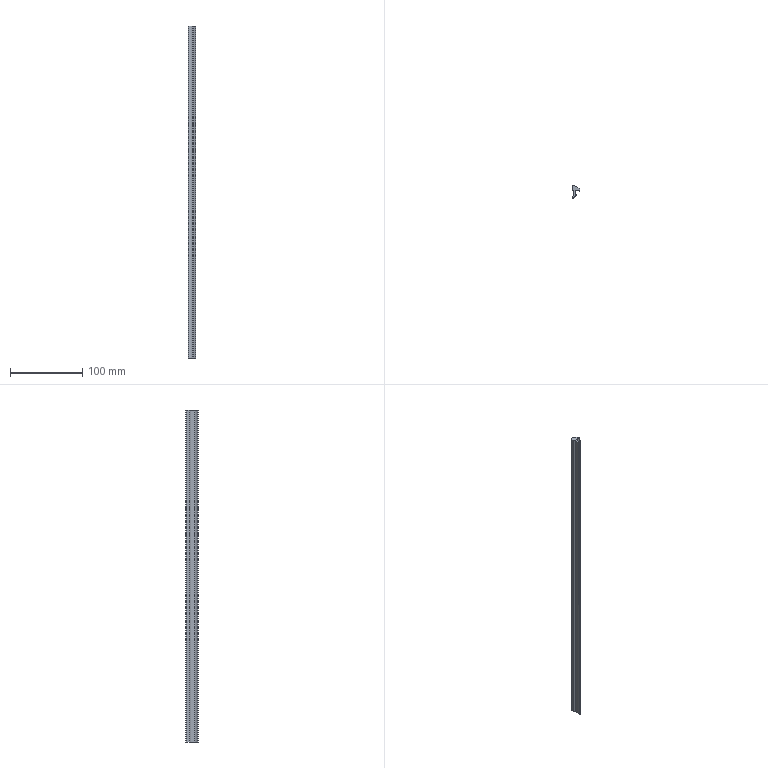Part | SolidWorks | features BaseBody 1, MoveFace 1 | 1 solid | 20 faces | box 10.8 x 17.5 x 461 mm | volume 36327 mm3 | cylinder 11 | plane 9 | commonest cylinder face diameters 1.6 x2 14 x2 0.4 x1 0.6 x1 0.8 x1 2.6 x1
STEP:
#1=CARTESIAN_POINT('',(-3.236,-11.055,361.));
#2=VERTEX_POINT('',#1);
#3=CARTESIAN_POINT('',(-4.3,-10.3,361.));
#4=VERTEX_POINT('',#3);
#5=CARTESIAN_POINT('',(-3.5,-10.3,361.));
#6=DIRECTION('',(0.,0.,-1.));
#7=DIRECTION('',(1.,0.,0.));
#8=AXIS2_PLACEMENT_3D('',#5,#6,#7);
#9=CIRCLE('',#8,0.8);
#10=EDGE_CURVE('',#2,#4,#9,.T.);
#11=ORIENTED_EDGE('',*,*,#10,.T.);
#12=CARTESIAN_POINT('',(-4.3,-10.3,-100.));
#13=VERTEX_POINT('',#12);
#14=CARTESIAN_POINT('',(-4.3,-10.3,-100.));
#15=DIRECTION('',(0.,0.,-1.));
#16=VECTOR('',#15,1000.);
#17=LINE('',#14,#16);
#18=EDGE_CURVE('',#4,#13,#17,.T.);
#19=ORIENTED_EDGE('',*,*,#18,.T.);
#20=CARTESIAN_POINT('',(-3.236,-11.055,-100.));
#21=VERTEX_POINT('',#20);
#22=CARTESIAN_POINT('',(-3.5,-10.3,-100.));
#23=DIRECTION('',(0.,0.,1.));
#24=DIRECTION('',(-1.,0.,0.));
#25=AXIS2_PLACEMENT_3D('',#22,#23,#24);
#26=CIRCLE('',#25,0.8);
#27=EDGE_CURVE('',#13,#21,#26,.T.);
#28=ORIENTED_EDGE('',*,*,#27,.T.);
#29=CARTESIAN_POINT('',(-3.236,-11.055,-100.));
#30=DIRECTION('',(0.,0.,-1.));
#31=VECTOR('',#30,1000.);
#32=LINE('',#29,#31);
#33=EDGE_CURVE('',#2,#21,#32,.T.);
#34=ORIENTED_EDGE('',*,*,#33,.F.);
#35=EDGE_LOOP('',(#11,#19,#28,#34));
#36=FACE_OUTER_BOUND('',#35,.T.);
#37=CARTESIAN_POINT('',(-3.5,-10.3,-100.));
#38=DIRECTION('',(0.,0.,-1.));
#39=DIRECTION('',(-1.,0.,0.));
#40=AXIS2_PLACEMENT_3D('',#37,#38,#39);
#41=CYLINDRICAL_SURFACE('',#40,0.8);
#42=ADVANCED_FACE('',(#36),#41,.T.);
#43=CARTESIAN_POINT('',(1.184,-6.397,-100.));
#44=VERTEX_POINT('',#43);
#45=CARTESIAN_POINT('',(-5.702,-4.29,-100.));
#46=DIRECTION('',(0.,0.,1.));
#47=DIRECTION('',(-1.,0.,0.));
#48=AXIS2_PLACEMENT_3D('',#45,#46,#47);
#49=CIRCLE('',#48,7.201);
#50=EDGE_CURVE('',#21,#44,#49,.T.);
#51=ORIENTED_EDGE('',*,*,#50,.T.);
#52=CARTESIAN_POINT('',(1.184,-6.397,361.));
#53=VERTEX_POINT('',#52);
#54=CARTESIAN_POINT('',(1.184,-6.397,-100.));
#55=DIRECTION('',(0.,0.,1.));
#56=VECTOR('',#55,1000.);
#57=LINE('',#54,#56);
#58=EDGE_CURVE('',#44,#53,#57,.T.);
#59=ORIENTED_EDGE('',*,*,#58,.T.);
#60=CARTESIAN_POINT('',(-5.702,-4.29,361.));
#61=DIRECTION('',(0.,0.,-1.));
#62=DIRECTION('',(1.,0.,0.));
#63=AXIS2_PLACEMENT_3D('',#60,#61,#62);
#64=CIRCLE('',#63,7.201);
#65=EDGE_CURVE('',#53,#2,#64,.T.);
#66=ORIENTED_EDGE('',*,*,#65,.T.);
#67=ORIENTED_EDGE('',*,*,#33,.T.);
#68=EDGE_LOOP('',(#51,#59,#66,#67));
#69=FACE_OUTER_BOUND('',#68,.T.);
#70=CARTESIAN_POINT('',(-5.702,-4.29,-100.));
#71=DIRECTION('',(0.,0.,-1.));
#72=DIRECTION('',(-1.,0.,0.));
#73=AXIS2_PLACEMENT_3D('',#70,#71,#72);
#74=CYLINDRICAL_SURFACE('',#73,7.201);
#75=ADVANCED_FACE('',(#69),#74,.T.);
#76=CARTESIAN_POINT('',(0.9,-6.,-100.));
#77=VERTEX_POINT('',#76);
#78=CARTESIAN_POINT('',(0.9,-6.3,-100.));
#79=DIRECTION('',(0.,0.,1.));
#80=DIRECTION('',(-1.,0.,0.));
#81=AXIS2_PLACEMENT_3D('',#78,#79,#80);
#82=CIRCLE('',#81,0.3);
#83=EDGE_CURVE('',#44,#77,#82,.T.);
#84=ORIENTED_EDGE('',*,*,#83,.T.);
#85=CARTESIAN_POINT('',(0.9,-6.,361.));
#86=VERTEX_POINT('',#85);
#87=CARTESIAN_POINT('',(0.9,-6.,-100.));
#88=DIRECTION('',(0.,0.,1.));
#89=VECTOR('',#88,1000.);
#90=LINE('',#87,#89);
#91=EDGE_CURVE('',#77,#86,#90,.T.);
#92=ORIENTED_EDGE('',*,*,#91,.T.);
#93=CARTESIAN_POINT('',(0.9,-6.3,361.));
#94=DIRECTION('',(0.,0.,-1.));
#95=DIRECTION('',(1.,0.,0.));
#96=AXIS2_PLACEMENT_3D('',#93,#94,#95);
#97=CIRCLE('',#96,0.3);
#98=EDGE_CURVE('',#86,#53,#97,.T.);
#99=ORIENTED_EDGE('',*,*,#98,.T.);
#100=ORIENTED_EDGE('',*,*,#58,.F.);
#101=EDGE_LOOP('',(#84,#92,#99,#100));
#102=FACE_OUTER_BOUND('',#101,.T.);
#103=CARTESIAN_POINT('',(0.9,-6.3,-100.));
#104=DIRECTION('',(0.,0.,-1.));
#105=DIRECTION('',(-1.,0.,0.));
#106=AXIS2_PLACEMENT_3D('',#103,#104,#105);
#107=CYLINDRICAL_SURFACE('',#106,0.3);
#108=ADVANCED_FACE('',(#102),#107,.T.);
#109=CARTESIAN_POINT('',(-2.5,-0.5,-100.));
#110=VERTEX_POINT('',#109);
#111=CARTESIAN_POINT('',(-2.5,-6.153,-100.));
#112=VERTEX_POINT('',#111);
#113=CARTESIAN_POINT('',(-2.5,-6.397,-100.));
#114=DIRECTION('',(0.,-1.,0.));
#115=VECTOR('',#114,1000.);
#116=LINE('',#113,#115);
#117=EDGE_CURVE('',#110,#112,#116,.T.);
#118=ORIENTED_EDGE('',*,*,#117,.F.);
#119=CARTESIAN_POINT('',(-4.2,1.695,-100.));
#120=VERTEX_POINT('',#119);
#121=CARTESIAN_POINT('',(-1.701,1.875,-100.));
#122=DIRECTION('',(0.,0.,1.));
#123=DIRECTION('',(-1.,0.,0.));
#124=AXIS2_PLACEMENT_3D('',#121,#122,#123);
#125=CIRCLE('',#124,2.506);
#126=EDGE_CURVE('',#120,#110,#125,.T.);
#127=ORIENTED_EDGE('',*,*,#126,.F.);
#128=CARTESIAN_POINT('',(-4.2,5.1,-100.));
#129=VERTEX_POINT('',#128);
#130=CARTESIAN_POINT('',(-4.2,-6.397,-100.));
#131=DIRECTION('',(0.,-1.,0.));
#132=VECTOR('',#131,1000.);
#133=LINE('',#130,#132);
#134=EDGE_CURVE('',#129,#120,#133,.T.);
#135=ORIENTED_EDGE('',*,*,#134,.F.);
#136=CARTESIAN_POINT('',(-2.892,6.4,-100.));
#137=VERTEX_POINT('',#136);
#138=CARTESIAN_POINT('',(-2.9,5.1,-100.));
#139=DIRECTION('',(0.,0.,1.));
#140=DIRECTION('',(-1.,0.,0.));
#141=AXIS2_PLACEMENT_3D('',#138,#139,#140);
#142=CIRCLE('',#141,1.3);
#143=EDGE_CURVE('',#137,#129,#142,.T.);
#144=ORIENTED_EDGE('',*,*,#143,.F.);
#145=CARTESIAN_POINT('',(0.5,5.5,-100.));
#146=VERTEX_POINT('',#145);
#147=CARTESIAN_POINT('',(-2.934,-0.5999,-100.));
#148=DIRECTION('',(0.,0.,1.));
#149=DIRECTION('',(-1.,0.,0.));
#150=AXIS2_PLACEMENT_3D('',#147,#148,#149);
#151=CIRCLE('',#150,7.);
#152=EDGE_CURVE('',#146,#137,#151,.T.);
#153=ORIENTED_EDGE('',*,*,#152,.F.);
#154=CARTESIAN_POINT('',(5.5,1.7,-100.));
#155=VERTEX_POINT('',#154);
#156=CARTESIAN_POINT('',(5.5,1.7,-100.));
#157=DIRECTION('',(-0.7962,0.6051,0.));
#158=VECTOR('',#157,1000.);
#159=LINE('',#156,#158);
#160=EDGE_CURVE('',#155,#146,#159,.T.);
#161=ORIENTED_EDGE('',*,*,#160,.F.);
#162=CARTESIAN_POINT('',(6.458,-0.2215,-100.));
#163=VERTEX_POINT('',#162);
#164=CARTESIAN_POINT('',(6.458,-0.2215,-100.));
#165=DIRECTION('',(-0.4462,0.8949,0.));
#166=VECTOR('',#165,1000.);
#167=LINE('',#164,#166);
#168=EDGE_CURVE('',#163,#155,#167,.T.);
#169=ORIENTED_EDGE('',*,*,#168,.F.);
#170=CARTESIAN_POINT('',(5.895,-0.7433,-100.));
#171=VERTEX_POINT('',#170);
#172=CARTESIAN_POINT('',(6.1,-0.4,-100.));
#173=DIRECTION('',(0.,0.,1.));
#174=DIRECTION('',(-1.,0.,0.));
#175=AXIS2_PLACEMENT_3D('',#172,#173,#174);
#176=CIRCLE('',#175,0.4);
#177=EDGE_CURVE('',#171,#163,#176,.T.);
#178=ORIENTED_EDGE('',*,*,#177,.F.);
#179=CARTESIAN_POINT('',(3.,0.,-100.));
#180=VERTEX_POINT('',#179);
#181=CARTESIAN_POINT('',(2.746,-6.995,-100.));
#182=DIRECTION('',(0.,0.,-1.));
#183=DIRECTION('',(-1.,0.,0.));
#184=AXIS2_PLACEMENT_3D('',#181,#182,#183);
#185=CIRCLE('',#184,7.);
#186=EDGE_CURVE('',#180,#171,#185,.T.);
#187=ORIENTED_EDGE('',*,*,#186,.F.);
#188=CARTESIAN_POINT('',(0.,0.,-100.));
#189=VERTEX_POINT('',#188);
#190=CARTESIAN_POINT('',(-6.814,0.,-100.));
#191=DIRECTION('',(1.,0.,0.));
#192=VECTOR('',#191,1000.);
#193=LINE('',#190,#192);
#194=EDGE_CURVE('',#189,#180,#193,.T.);
#195=ORIENTED_EDGE('',*,*,#194,.F.);
#196=CARTESIAN_POINT('',(0.,-5.8,-100.));
#197=VERTEX_POINT('',#196);
#198=CARTESIAN_POINT('',(0.,-6.397,-100.));
#199=DIRECTION('',(0.,1.,0.));
#200=VECTOR('',#199,1000.);
#201=LINE('',#198,#200);
#202=EDGE_CURVE('',#197,#189,#201,.T.);
#203=ORIENTED_EDGE('',*,*,#202,.F.);
#204=CARTESIAN_POINT('',(0.2,-6.,-100.));
#205=VERTEX_POINT('',#204);
#206=CARTESIAN_POINT('',(0.2,-5.8,-100.));
#207=DIRECTION('',(0.,0.,1.));
#208=DIRECTION('',(-1.,0.,0.));
#209=AXIS2_PLACEMENT_3D('',#206,#207,#208);
#210=CIRCLE('',#209,0.2);
#211=EDGE_CURVE('',#197,#205,#210,.T.);
#212=ORIENTED_EDGE('',*,*,#211,.T.);
#213=CARTESIAN_POINT('',(-6.814,-6.,-100.));
#214=DIRECTION('',(-1.,0.,0.));
#215=VECTOR('',#214,1000.);
#216=LINE('',#213,#215);
#217=EDGE_CURVE('',#77,#205,#216,.T.);
#218=ORIENTED_EDGE('',*,*,#217,.F.);
#219=ORIENTED_EDGE('',*,*,#83,.F.);
#220=ORIENTED_EDGE('',*,*,#50,.F.);
#221=ORIENTED_EDGE('',*,*,#27,.F.);
#222=CARTESIAN_POINT('',(-3.998,-9.674,-100.));
#223=VERTEX_POINT('',#222);
#224=CARTESIAN_POINT('',(-3.5,-10.3,-100.));
#225=DIRECTION('',(0.,0.,1.));
#226=DIRECTION('',(-1.,0.,0.));
#227=AXIS2_PLACEMENT_3D('',#224,#225,#226);
#228=CIRCLE('',#227,0.8);
#229=EDGE_CURVE('',#223,#13,#228,.T.);
#230=ORIENTED_EDGE('',*,*,#229,.F.);
#231=CARTESIAN_POINT('',(-6.814,-6.397,-100.));
#232=DIRECTION('',(0.,0.,-1.));
#233=DIRECTION('',(-1.,0.,0.));
#234=AXIS2_PLACEMENT_3D('',#231,#232,#233);
#235=CIRCLE('',#234,4.321);
#236=EDGE_CURVE('',#112,#223,#235,.T.);
#237=ORIENTED_EDGE('',*,*,#236,.F.);
#238=EDGE_LOOP('',(#118,#127,#135,#144,#153,#161,#169,#178,#187,#195,#203,#212,#218,#219,#220,#221,#230,#237));
#239=FACE_OUTER_BOUND('',#238,.T.);
#240=CARTESIAN_POINT('',(-6.814,-6.397,-100.));
#241=DIRECTION('',(0.,0.,1.));
#242=DIRECTION('',(1.,0.,0.));
#243=AXIS2_PLACEMENT_3D('',#240,#241,#242);
#244=PLANE('',#243);
#245=ADVANCED_FACE('',(#239),#244,.F.);
#246=ORIENTED_EDGE('',*,*,#18,.F.);
#247=CARTESIAN_POINT('',(-3.998,-9.674,361.));
#248=VERTEX_POINT('',#247);
#249=CARTESIAN_POINT('',(-3.5,-10.3,361.));
#250=DIRECTION('',(0.,0.,-1.));
#251=DIRECTION('',(1.,0.,0.));
#252=AXIS2_PLACEMENT_3D('',#249,#250,#251);
#253=CIRCLE('',#252,0.8);
#254=EDGE_CURVE('',#4,#248,#253,.T.);
#255=ORIENTED_EDGE('',*,*,#254,.T.);
#256=CARTESIAN_POINT('',(-3.998,-9.674,-100.));
#257=DIRECTION('',(0.,0.,-1.));
#258=VECTOR('',#257,1000.);
#259=LINE('',#256,#258);
#260=EDGE_CURVE('',#248,#223,#259,.T.);
#261=ORIENTED_EDGE('',*,*,#260,.T.);
#262=ORIENTED_EDGE('',*,*,#229,.T.);
#263=EDGE_LOOP('',(#246,#255,#261,#262));
#264=FACE_OUTER_BOUND('',#263,.T.);
#265=CARTESIAN_POINT('',(-3.5,-10.3,-100.));
#266=DIRECTION('',(0.,0.,-1.));
#267=DIRECTION('',(-1.,0.,0.));
#268=AXIS2_PLACEMENT_3D('',#265,#266,#267);
#269=CYLINDRICAL_SURFACE('',#268,0.8);
#270=ADVANCED_FACE('',(#264),#269,.T.);
#271=CARTESIAN_POINT('',(-4.2,1.695,361.));
#272=VERTEX_POINT('',#271);
#273=CARTESIAN_POINT('',(-2.5,-0.5,361.));
#274=VERTEX_POINT('',#273);
#275=CARTESIAN_POINT('',(-1.701,1.875,361.));
#276=DIRECTION('',(0.,0.,1.));
#277=DIRECTION('',(1.,0.,0.));
#278=AXIS2_PLACEMENT_3D('',#275,#276,#277);
#279=CIRCLE('',#278,2.506);
#280=EDGE_CURVE('',#272,#274,#279,.T.);
#281=ORIENTED_EDGE('',*,*,#280,.T.);
#282=CARTESIAN_POINT('',(-2.5,-6.153,361.));
#283=VERTEX_POINT('',#282);
#284=CARTESIAN_POINT('',(-2.5,-6.397,361.));
#285=DIRECTION('',(0.,-1.,0.));
#286=VECTOR('',#285,1000.);
#287=LINE('',#284,#286);
#288=EDGE_CURVE('',#274,#283,#287,.T.);
#289=ORIENTED_EDGE('',*,*,#288,.T.);
#290=CARTESIAN_POINT('',(-6.814,-6.397,361.));
#291=DIRECTION('',(0.,0.,-1.));
#292=DIRECTION('',(1.,0.,0.));
#293=AXIS2_PLACEMENT_3D('',#290,#291,#292);
#294=CIRCLE('',#293,4.321);
#295=EDGE_CURVE('',#283,#248,#294,.T.);
#296=ORIENTED_EDGE('',*,*,#295,.T.);
#297=ORIENTED_EDGE('',*,*,#254,.F.);
#298=ORIENTED_EDGE('',*,*,#10,.F.);
#299=ORIENTED_EDGE('',*,*,#65,.F.);
#300=ORIENTED_EDGE('',*,*,#98,.F.);
#301=CARTESIAN_POINT('',(0.2,-6.,361.));
#302=VERTEX_POINT('',#301);
#303=CARTESIAN_POINT('',(-6.814,-6.,361.));
#304=DIRECTION('',(-1.,0.,0.));
#305=VECTOR('',#304,1000.);
#306=LINE('',#303,#305);
#307=EDGE_CURVE('',#86,#302,#306,.T.);
#308=ORIENTED_EDGE('',*,*,#307,.T.);
#309=CARTESIAN_POINT('',(0.,-5.8,361.));
#310=VERTEX_POINT('',#309);
#311=CARTESIAN_POINT('',(0.2,-5.8,361.));
#312=DIRECTION('',(0.,0.,-1.));
#313=DIRECTION('',(1.,0.,0.));
#314=AXIS2_PLACEMENT_3D('',#311,#312,#313);
#315=CIRCLE('',#314,0.2);
#316=EDGE_CURVE('',#302,#310,#315,.T.);
#317=ORIENTED_EDGE('',*,*,#316,.T.);
#318=CARTESIAN_POINT('',(0.,0.,361.));
#319=VERTEX_POINT('',#318);
#320=CARTESIAN_POINT('',(0.,-6.397,361.));
#321=DIRECTION('',(0.,1.,0.));
#322=VECTOR('',#321,1000.);
#323=LINE('',#320,#322);
#324=EDGE_CURVE('',#310,#319,#323,.T.);
#325=ORIENTED_EDGE('',*,*,#324,.T.);
#326=CARTESIAN_POINT('',(3.,0.,361.));
#327=VERTEX_POINT('',#326);
#328=CARTESIAN_POINT('',(-6.814,0.,361.));
#329=DIRECTION('',(1.,0.,0.));
#330=VECTOR('',#329,1000.);
#331=LINE('',#328,#330);
#332=EDGE_CURVE('',#319,#327,#331,.T.);
#333=ORIENTED_EDGE('',*,*,#332,.T.);
#334=CARTESIAN_POINT('',(5.895,-0.7433,361.));
#335=VERTEX_POINT('',#334);
#336=CARTESIAN_POINT('',(2.746,-6.995,361.));
#337=DIRECTION('',(0.,0.,-1.));
#338=DIRECTION('',(1.,0.,0.));
#339=AXIS2_PLACEMENT_3D('',#336,#337,#338);
#340=CIRCLE('',#339,7.);
#341=EDGE_CURVE('',#327,#335,#340,.T.);
#342=ORIENTED_EDGE('',*,*,#341,.T.);
#343=CARTESIAN_POINT('',(6.458,-0.2215,361.));
#344=VERTEX_POINT('',#343);
#345=CARTESIAN_POINT('',(6.1,-0.4,361.));
#346=DIRECTION('',(0.,0.,-1.));
#347=DIRECTION('',(1.,0.,0.));
#348=AXIS2_PLACEMENT_3D('',#345,#346,#347);
#349=CIRCLE('',#348,0.4);
#350=EDGE_CURVE('',#344,#335,#349,.T.);
#351=ORIENTED_EDGE('',*,*,#350,.F.);
#352=CARTESIAN_POINT('',(5.5,1.7,361.));
#353=VERTEX_POINT('',#352);
#354=CARTESIAN_POINT('',(6.282,0.1323,361.));
#355=DIRECTION('',(-0.4462,0.8949,0.));
#356=VECTOR('',#355,1000.);
#357=LINE('',#354,#356);
#358=EDGE_CURVE('',#344,#353,#357,.T.);
#359=ORIENTED_EDGE('',*,*,#358,.T.);
#360=CARTESIAN_POINT('',(0.5,5.5,361.));
#361=VERTEX_POINT('',#360);
#362=CARTESIAN_POINT('',(1.595,4.668,361.));
#363=DIRECTION('',(-0.7962,0.6051,0.));
#364=VECTOR('',#363,1000.);
#365=LINE('',#362,#364);
#366=EDGE_CURVE('',#353,#361,#365,.T.);
#367=ORIENTED_EDGE('',*,*,#366,.T.);
#368=CARTESIAN_POINT('',(-2.892,6.4,361.));
#369=VERTEX_POINT('',#368);
#370=CARTESIAN_POINT('',(-2.934,-0.5999,361.));
#371=DIRECTION('',(0.,0.,1.));
#372=DIRECTION('',(1.,0.,0.));
#373=AXIS2_PLACEMENT_3D('',#370,#371,#372);
#374=CIRCLE('',#373,7.);
#375=EDGE_CURVE('',#361,#369,#374,.T.);
#376=ORIENTED_EDGE('',*,*,#375,.T.);
#377=CARTESIAN_POINT('',(-4.2,5.1,361.));
#378=VERTEX_POINT('',#377);
#379=CARTESIAN_POINT('',(-2.9,5.1,361.));
#380=DIRECTION('',(0.,0.,1.));
#381=DIRECTION('',(1.,0.,0.));
#382=AXIS2_PLACEMENT_3D('',#379,#380,#381);
#383=CIRCLE('',#382,1.3);
#384=EDGE_CURVE('',#369,#378,#383,.T.);
#385=ORIENTED_EDGE('',*,*,#384,.T.);
#386=CARTESIAN_POINT('',(-4.2,-6.397,361.));
#387=DIRECTION('',(0.,-1.,0.));
#388=VECTOR('',#387,1000.);
#389=LINE('',#386,#388);
#390=EDGE_CURVE('',#378,#272,#389,.T.);
#391=ORIENTED_EDGE('',*,*,#390,.T.);
#392=EDGE_LOOP('',(#281,#289,#296,#297,#298,#299,#300,#308,#317,#325,#333,#342,#351,#359,#367,#376,#385,#391));
#393=FACE_OUTER_BOUND('',#392,.T.);
#394=CARTESIAN_POINT('',(-6.814,-6.397,361.));
#395=DIRECTION('',(0.,0.,1.));
#396=DIRECTION('',(1.,0.,0.));
#397=AXIS2_PLACEMENT_3D('',#394,#395,#396);
#398=PLANE('',#397);
#399=ADVANCED_FACE('',(#393),#398,.T.);
#400=ORIENTED_EDGE('',*,*,#217,.T.);
#401=CARTESIAN_POINT('',(0.2,-6.,-100.));
#402=DIRECTION('',(0.,0.,1.));
#403=VECTOR('',#402,1000.);
#404=LINE('',#401,#403);
#405=EDGE_CURVE('',#205,#302,#404,.T.);
#406=ORIENTED_EDGE('',*,*,#405,.T.);
#407=ORIENTED_EDGE('',*,*,#307,.F.);
#408=ORIENTED_EDGE('',*,*,#91,.F.);
#409=EDGE_LOOP('',(#400,#406,#407,#408));
#410=FACE_OUTER_BOUND('',#409,.T.);
#411=CARTESIAN_POINT('',(0.9,-6.,-100.));
#412=DIRECTION('',(0.,1.,0.));
#413=DIRECTION('',(0.,0.,1.));
#414=AXIS2_PLACEMENT_3D('',#411,#412,#413);
#415=PLANE('',#414);
#416=ADVANCED_FACE('',(#410),#415,.T.);
#417=CARTESIAN_POINT('',(-2.5,-6.153,-100.));
#418=DIRECTION('',(0.,0.,1.));
#419=VECTOR('',#418,1000.);
#420=LINE('',#417,#419);
#421=EDGE_CURVE('',#112,#283,#420,.T.);
#422=ORIENTED_EDGE('',*,*,#421,.F.);
#423=ORIENTED_EDGE('',*,*,#236,.T.);
#424=ORIENTED_EDGE('',*,*,#260,.F.);
#425=ORIENTED_EDGE('',*,*,#295,.F.);
#426=EDGE_LOOP('',(#422,#423,#424,#425));
#427=FACE_OUTER_BOUND('',#426,.T.);
#428=CARTESIAN_POINT('',(-6.814,-6.397,-100.));
#429=DIRECTION('',(0.,0.,-1.));
#430=DIRECTION('',(-1.,0.,0.));
#431=AXIS2_PLACEMENT_3D('',#428,#429,#430);
#432=CYLINDRICAL_SURFACE('',#431,4.321);
#433=ADVANCED_FACE('',(#427),#432,.F.);
#434=ORIENTED_EDGE('',*,*,#117,.T.);
#435=ORIENTED_EDGE('',*,*,#421,.T.);
#436=ORIENTED_EDGE('',*,*,#288,.F.);
#437=CARTESIAN_POINT('',(-2.5,-0.5,-100.));
#438=DIRECTION('',(0.,0.,-1.));
#439=VECTOR('',#438,1000.);
#440=LINE('',#437,#439);
#441=EDGE_CURVE('',#274,#110,#440,.T.);
#442=ORIENTED_EDGE('',*,*,#441,.T.);
#443=EDGE_LOOP('',(#434,#435,#436,#442));
#444=FACE_OUTER_BOUND('',#443,.T.);
#445=CARTESIAN_POINT('',(-2.5,-0.5,-100.));
#446=DIRECTION('',(-1.,0.,0.));
#447=DIRECTION('',(0.,0.,1.));
#448=AXIS2_PLACEMENT_3D('',#445,#446,#447);
#449=PLANE('',#448);
#450=ADVANCED_FACE('',(#444),#449,.T.);
#451=ORIENTED_EDGE('',*,*,#126,.T.);
#452=ORIENTED_EDGE('',*,*,#441,.F.);
#453=ORIENTED_EDGE('',*,*,#280,.F.);
#454=CARTESIAN_POINT('',(-4.2,1.695,-100.));
#455=DIRECTION('',(0.,0.,-1.));
#456=VECTOR('',#455,1000.);
#457=LINE('',#454,#456);
#458=EDGE_CURVE('',#272,#120,#457,.T.);
#459=ORIENTED_EDGE('',*,*,#458,.T.);
#460=EDGE_LOOP('',(#451,#452,#453,#459));
#461=FACE_OUTER_BOUND('',#460,.T.);
#462=CARTESIAN_POINT('',(-1.701,1.875,-100.));
#463=DIRECTION('',(0.,0.,-1.));
#464=DIRECTION('',(-1.,0.,0.));
#465=AXIS2_PLACEMENT_3D('',#462,#463,#464);
#466=CYLINDRICAL_SURFACE('',#465,2.506);
#467=ADVANCED_FACE('',(#461),#466,.T.);
#468=ORIENTED_EDGE('',*,*,#134,.T.);
#469=ORIENTED_EDGE('',*,*,#458,.F.);
#470=ORIENTED_EDGE('',*,*,#390,.F.);
#471=CARTESIAN_POINT('',(-4.2,5.1,-100.));
#472=DIRECTION('',(0.,0.,-1.));
#473=VECTOR('',#472,1000.);
#474=LINE('',#471,#473);
#475=EDGE_CURVE('',#378,#129,#474,.T.);
#476=ORIENTED_EDGE('',*,*,#475,.T.);
#477=EDGE_LOOP('',(#468,#469,#470,#476));
#478=FACE_OUTER_BOUND('',#477,.T.);
#479=CARTESIAN_POINT('',(-4.2,5.1,-100.));
#480=DIRECTION('',(-1.,0.,0.));
#481=DIRECTION('',(0.,0.,1.));
#482=AXIS2_PLACEMENT_3D('',#479,#480,#481);
#483=PLANE('',#482);
#484=ADVANCED_FACE('',(#478),#483,.T.);
#485=ORIENTED_EDGE('',*,*,#143,.T.);
#486=ORIENTED_EDGE('',*,*,#475,.F.);
#487=ORIENTED_EDGE('',*,*,#384,.F.);
#488=CARTESIAN_POINT('',(-2.892,6.4,-100.));
#489=DIRECTION('',(0.,0.,-1.));
#490=VECTOR('',#489,1000.);
#491=LINE('',#488,#490);
#492=EDGE_CURVE('',#369,#137,#491,.T.);
#493=ORIENTED_EDGE('',*,*,#492,.T.);
#494=EDGE_LOOP('',(#485,#486,#487,#493));
#495=FACE_OUTER_BOUND('',#494,.T.);
#496=CARTESIAN_POINT('',(-2.9,5.1,-100.));
#497=DIRECTION('',(0.,0.,-1.));
#498=DIRECTION('',(-1.,0.,0.));
#499=AXIS2_PLACEMENT_3D('',#496,#497,#498);
#500=CYLINDRICAL_SURFACE('',#499,1.3);
#501=ADVANCED_FACE('',(#495),#500,.T.);
#502=ORIENTED_EDGE('',*,*,#152,.T.);
#503=ORIENTED_EDGE('',*,*,#492,.F.);
#504=ORIENTED_EDGE('',*,*,#375,.F.);
#505=CARTESIAN_POINT('',(0.5,5.5,-100.));
#506=DIRECTION('',(0.,0.,-1.));
#507=VECTOR('',#506,1000.);
#508=LINE('',#505,#507);
#509=EDGE_CURVE('',#361,#146,#508,.T.);
#510=ORIENTED_EDGE('',*,*,#509,.T.);
#511=EDGE_LOOP('',(#502,#503,#504,#510));
#512=FACE_OUTER_BOUND('',#511,.T.);
#513=CARTESIAN_POINT('',(-2.934,-0.5999,-100.));
#514=DIRECTION('',(0.,0.,-1.));
#515=DIRECTION('',(-1.,0.,0.));
#516=AXIS2_PLACEMENT_3D('',#513,#514,#515);
#517=CYLINDRICAL_SURFACE('',#516,7.);
#518=ADVANCED_FACE('',(#512),#517,.T.);
#519=ORIENTED_EDGE('',*,*,#160,.T.);
#520=ORIENTED_EDGE('',*,*,#509,.F.);
#521=ORIENTED_EDGE('',*,*,#366,.F.);
#522=CARTESIAN_POINT('',(5.5,1.7,-100.));
#523=DIRECTION('',(0.,0.,-1.));
#524=VECTOR('',#523,1000.);
#525=LINE('',#522,#524);
#526=EDGE_CURVE('',#353,#155,#525,.T.);
#527=ORIENTED_EDGE('',*,*,#526,.T.);
#528=EDGE_LOOP('',(#519,#520,#521,#527));
#529=FACE_OUTER_BOUND('',#528,.T.);
#530=CARTESIAN_POINT('',(5.5,1.7,-100.));
#531=DIRECTION('',(0.6051,0.7962,0.));
#532=DIRECTION('',(-0.7962,0.6051,0.));
#533=AXIS2_PLACEMENT_3D('',#530,#531,#532);
#534=PLANE('',#533);
#535=ADVANCED_FACE('',(#529),#534,.T.);
#536=ORIENTED_EDGE('',*,*,#168,.T.);
#537=ORIENTED_EDGE('',*,*,#526,.F.);
#538=ORIENTED_EDGE('',*,*,#358,.F.);
#539=CARTESIAN_POINT('',(6.458,-0.2215,-100.));
#540=DIRECTION('',(0.,0.,-1.));
#541=VECTOR('',#540,1000.);
#542=LINE('',#539,#541);
#543=EDGE_CURVE('',#344,#163,#542,.T.);
#544=ORIENTED_EDGE('',*,*,#543,.T.);
#545=EDGE_LOOP('',(#536,#537,#538,#544));
#546=FACE_OUTER_BOUND('',#545,.T.);
#547=CARTESIAN_POINT('',(6.458,-0.2215,-100.));
#548=DIRECTION('',(0.8949,0.4462,0.));
#549=DIRECTION('',(-0.4462,0.8949,0.));
#550=AXIS2_PLACEMENT_3D('',#547,#548,#549);
#551=PLANE('',#550);
#552=ADVANCED_FACE('',(#546),#551,.T.);
#553=CARTESIAN_POINT('',(3.,0.,-100.));
#554=DIRECTION('',(0.,0.,1.));
#555=VECTOR('',#554,1000.);
#556=LINE('',#553,#555);
#557=EDGE_CURVE('',#180,#327,#556,.T.);
#558=ORIENTED_EDGE('',*,*,#557,.F.);
#559=ORIENTED_EDGE('',*,*,#186,.T.);
#560=CARTESIAN_POINT('',(5.895,-0.7433,-100.));
#561=DIRECTION('',(0.,0.,-1.));
#562=VECTOR('',#561,1000.);
#563=LINE('',#560,#562);
#564=EDGE_CURVE('',#335,#171,#563,.T.);
#565=ORIENTED_EDGE('',*,*,#564,.F.);
#566=ORIENTED_EDGE('',*,*,#341,.F.);
#567=EDGE_LOOP('',(#558,#559,#565,#566));
#568=FACE_OUTER_BOUND('',#567,.T.);
#569=CARTESIAN_POINT('',(2.746,-6.995,-100.));
#570=DIRECTION('',(0.,0.,-1.));
#571=DIRECTION('',(-1.,0.,0.));
#572=AXIS2_PLACEMENT_3D('',#569,#570,#571);
#573=CYLINDRICAL_SURFACE('',#572,7.);
#574=ADVANCED_FACE('',(#568),#573,.F.);
#575=ORIENTED_EDGE('',*,*,#194,.T.);
#576=ORIENTED_EDGE('',*,*,#557,.T.);
#577=ORIENTED_EDGE('',*,*,#332,.F.);
#578=CARTESIAN_POINT('',(0.,0.,-100.));
#579=DIRECTION('',(0.,0.,-1.));
#580=VECTOR('',#579,1000.);
#581=LINE('',#578,#580);
#582=EDGE_CURVE('',#319,#189,#581,.T.);
#583=ORIENTED_EDGE('',*,*,#582,.T.);
#584=EDGE_LOOP('',(#575,#576,#577,#583));
#585=FACE_OUTER_BOUND('',#584,.T.);
#586=CARTESIAN_POINT('',(0.,0.,-100.));
#587=DIRECTION('',(0.,-1.,0.));
#588=DIRECTION('',(0.,0.,-1.));
#589=AXIS2_PLACEMENT_3D('',#586,#587,#588);
#590=PLANE('',#589);
#591=ADVANCED_FACE('',(#585),#590,.T.);
#592=ORIENTED_EDGE('',*,*,#202,.T.);
#593=ORIENTED_EDGE('',*,*,#582,.F.);
#594=ORIENTED_EDGE('',*,*,#324,.F.);
#595=CARTESIAN_POINT('',(0.,-5.8,-100.));
#596=DIRECTION('',(0.,0.,-1.));
#597=VECTOR('',#596,1000.);
#598=LINE('',#595,#597);
#599=EDGE_CURVE('',#310,#197,#598,.T.);
#600=ORIENTED_EDGE('',*,*,#599,.T.);
#601=EDGE_LOOP('',(#592,#593,#594,#600));
#602=FACE_OUTER_BOUND('',#601,.T.);
#603=CARTESIAN_POINT('',(0.,-5.8,-100.));
#604=DIRECTION('',(1.,0.,0.));
#605=DIRECTION('',(0.,0.,-1.));
#606=AXIS2_PLACEMENT_3D('',#603,#604,#605);
#607=PLANE('',#606);
#608=ADVANCED_FACE('',(#602),#607,.T.);
#609=ORIENTED_EDGE('',*,*,#405,.F.);
#610=ORIENTED_EDGE('',*,*,#211,.F.);
#611=ORIENTED_EDGE('',*,*,#599,.F.);
#612=ORIENTED_EDGE('',*,*,#316,.F.);
#613=EDGE_LOOP('',(#609,#610,#611,#612));
#614=FACE_OUTER_BOUND('',#613,.T.);
#615=CARTESIAN_POINT('',(0.2,-5.8,-100.));
#616=DIRECTION('',(0.,0.,-1.));
#617=DIRECTION('',(-1.,0.,0.));
#618=AXIS2_PLACEMENT_3D('',#615,#616,#617);
#619=CYLINDRICAL_SURFACE('',#618,0.2);
#620=ADVANCED_FACE('',(#614),#619,.F.);
#621=ORIENTED_EDGE('',*,*,#177,.T.);
#622=ORIENTED_EDGE('',*,*,#543,.F.);
#623=ORIENTED_EDGE('',*,*,#350,.T.);
#624=ORIENTED_EDGE('',*,*,#564,.T.);
#625=EDGE_LOOP('',(#621,#622,#623,#624));
#626=FACE_OUTER_BOUND('',#625,.T.);
#627=CARTESIAN_POINT('',(6.1,-0.4,-100.));
#628=DIRECTION('',(0.,0.,-1.));
#629=DIRECTION('',(-1.,0.,0.));
#630=AXIS2_PLACEMENT_3D('',#627,#628,#629);
#631=CYLINDRICAL_SURFACE('',#630,0.4);
#632=ADVANCED_FACE('',(#626),#631,.T.);
#633=CLOSED_SHELL('',(#42,#75,#108,#245,#270,#399,#416,#433,#450,#467,#484,#501,#518,#535,#552,#574,#591,#608,#620,#632));
#634=MANIFOLD_SOLID_BREP('',#633);
#635=CARTESIAN_POINT('',(0.,0.,0.));
#636=DIRECTION('',(0.,0.,1.));
#637=DIRECTION('',(1.,0.,0.));
#638=AXIS2_PLACEMENT_3D('',#635,#636,#637);
#639=(LENGTH_UNIT()NAMED_UNIT(*)SI_UNIT(.MILLI.,.METRE.));
#640=UNCERTAINTY_MEASURE_WITH_UNIT(LENGTH_MEASURE(0.00001),#639,'','');
#641=(NAMED_UNIT(*)PLANE_ANGLE_UNIT()SI_UNIT($,.RADIAN.));
#642=(NAMED_UNIT(*)SI_UNIT($,.STERADIAN.)SOLID_ANGLE_UNIT());
#643=(GEOMETRIC_REPRESENTATION_CONTEXT(3)GLOBAL_UNCERTAINTY_ASSIGNED_CONTEXT((#640))GLOBAL_UNIT_ASSIGNED_CONTEXT((#639,#641,#642))REPRESENTATION_CONTEXT('',''));
#644=ADVANCED_BREP_SHAPE_REPRESENTATION('',(#634,#638),#643);